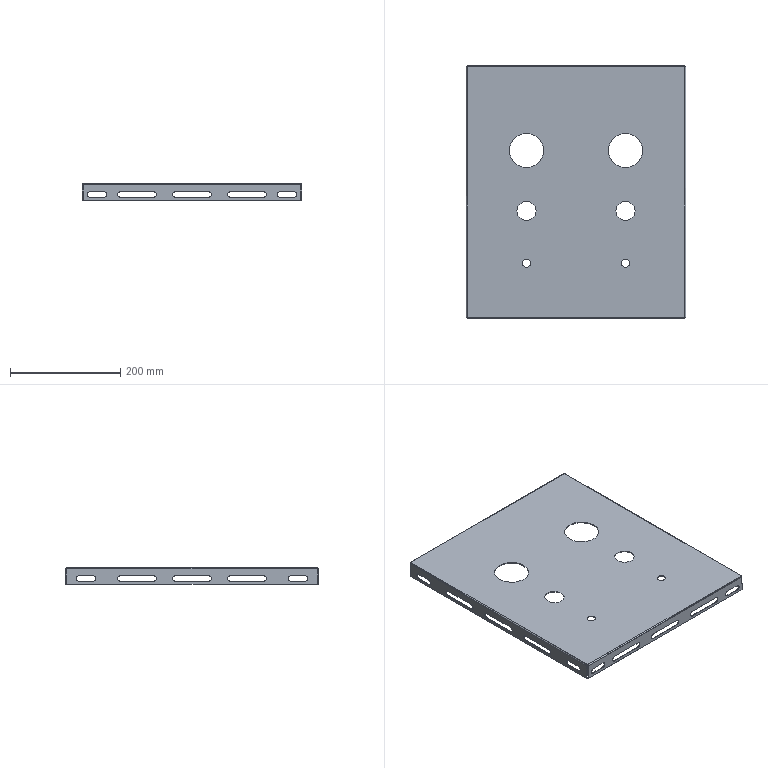Part | SolidWorks | features ICE 2, Cut 1, EdgeFlange 1, FlatPattern 1, SMBaseFlange 1, SheetMetal 1 | 1 solid | 130 faces | box 399 x 459 x 30 mm | volume 317293 mm3 | plane 62 | cylinder 60 | spline 8 | commonest cylinder face diameters 10 x40 1 x4 4 x4 15 x4 35 x4 62 x4